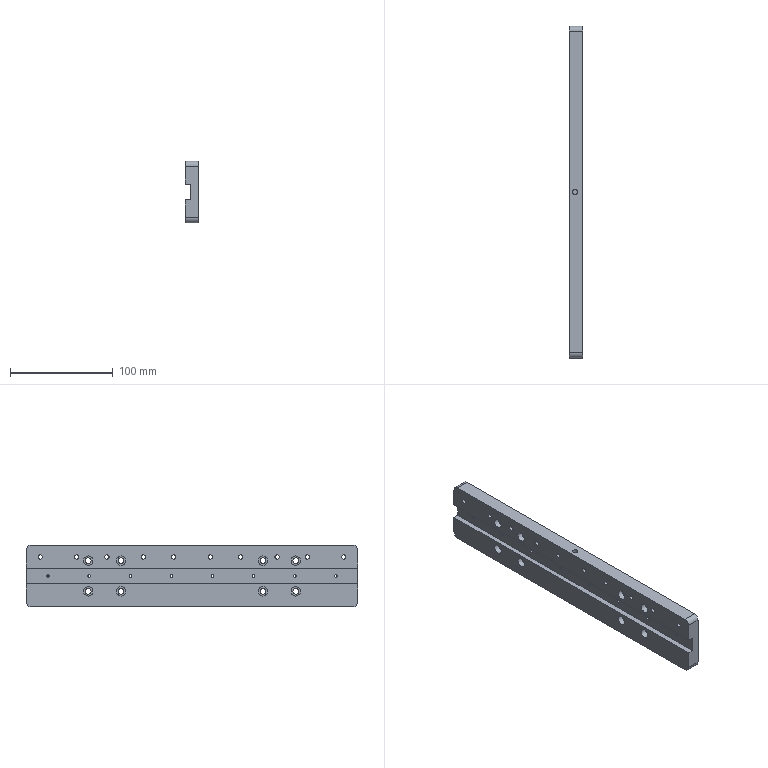Part | 1 solid | 58 faces | box 13 x 323 x 60 mm | volume 220136 mm3 | cylinder 39 | plane 19 | commonest cylinder face diameters 4.2 x10 2.5 x8 5.5 x8 9 x8 10 x4 5 x1